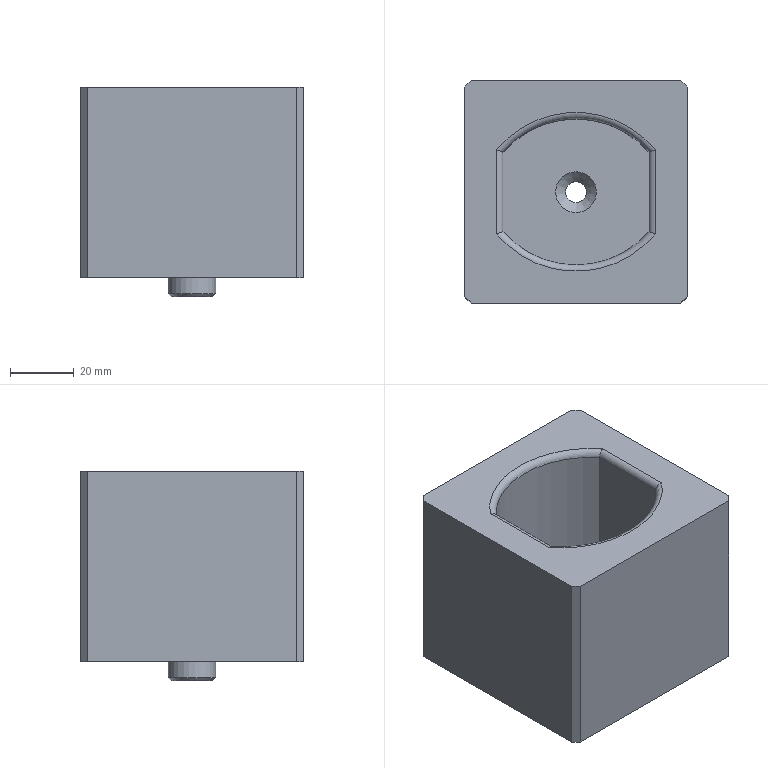NC program | NX | posted with a generic post | part box 70 x 70 x 66 mm
Whole program:
N10 G17 G21 G94 G90
(FLOOR_WALL , TOOL : D63)
N12 T01 M6
N14 G54
N16 G17 G0 G90 X-72.5 Y37.997 S6500 M3
N18 G43 Z30. H1
N20 Z3.
N22 G94 G1 Z0. F2500.
N24 X-69.5
N26 X69.5
N28 Y12.599
N30 X-69.5
N32 Y-12.8
N34 X69.5
N36 X72.5
N38 Z3.
N40 G0 Z30.
N42 M5
(DRILLING , TOOL : D8A45)
N44 T06 M6
N46 G54
N48 G17 G0 G90 X0. Y0. S5000 M3
N50 G43 Z30. H6
N52 G94 G81 G98 Z-3.4 F250. R3.
N54 G80
N56 G0 X0. Y0. Z30.
N58 M5
(DRILLING_COPY , TOOL : 6.6ZT)
N60 T16 M6
N62 G54
N64 G17 G0 G90 X0. Y0. S2000 M3
N66 G43 Z30. H16
N68 G94 G83 G98 Z-14.983 F250. Q2. R3.
N70 G80
N72 G0 X0. Y0. Z30.
N74 M5
(ZLEVEL_PROFILE , TOOL : D16)
N76 T22 M6
N78 G54
N80 G17 G0 G90 X-2.862 Y-43.15 S7500 M3
N82 G43 Z30. H22
N84 Z1.4
N86 G94 G1 X-33. Z-0.179 F1000.
N88 X-33.7 Z-0.216
N90 X-35.342 Y-42.838 Z-0.304
N92 X-36.886 Y-42.198 Z-0.391
N94 X-38.268 Y-41.258 Z-0.479
N96 X-41.258 Y-38.268 Z-0.701
N98 X-42.198 Y-36.886 Z-0.788
N100 X-42.838 Y-35.342 Z-0.876
N102 X-43.15 Y-33.7 Z-0.963
N104 Y-33. Z-1.
N106 Y33. F2500.
N108 G2 X-40.763 Y38.763 R8.15
N110 G1 X-38.763 Y40.763
N112 G2 X-33. Y43.15 R8.15
N114 G1 X33.
N116 G2 X38.763 Y40.763 R8.15
N118 G1 X40.763 Y38.763
N120 G2 X43.15 Y33. R8.15
N122 G1 Y-33.
N124 G2 X40.763 Y-38.763 R8.15
N126 G1 X38.763 Y-40.763
N128 G2 X33. Y-43.15 R8.15
N130 G1 X-33.
N132 G2 X-38.763 Y-40.763 R8.15
N134 G1 X-40.763 Y-38.763
N136 G2 X-43.15 Y-33. R8.15
N138 G1 Y24.29 Z-2.
N140 Y33.
N142 G2 X-40.763 Y38.763 R8.15
N144 G1 X-38.763 Y40.763
N146 G2 X-33. Y43.15 R8.15
N148 G1 X33.
N150 G2 X38.763 Y40.763 R8.15
N152 G1 X40.763 Y38.763
N154 G2 X43.15 Y33. R8.15
N156 G1 Y-33.
N158 G2 X40.763 Y-38.763 R8.15
N160 G1 X38.763 Y-40.763
N162 G2 X33. Y-43.15 R8.15
N164 G1 X-33.
N166 G2 X-38.763 Y-40.763 R8.15
N168 G1 X-40.763 Y-38.763
N170 G2 X-43.15 Y-33. R8.15
N172 G1 Y24.29 Z-3.
N174 Y33.
N176 G2 X-40.763 Y38.763 R8.15
N178 G1 X-38.763 Y40.763
N180 G2 X-33. Y43.15 R8.15
N182 G1 X33.
N184 G2 X38.763 Y40.763 R8.15
N186 G1 X40.763 Y38.763
N188 G2 X43.15 Y33. R8.15
N190 G1 Y-33.
N192 G2 X40.763 Y-38.763 R8.15
N194 G1 X38.763 Y-40.763
N196 G2 X33. Y-43.15 R8.15
N198 G1 X-33.
N200 G2 X-38.763 Y-40.763 R8.15
N202 G1 X-40.763 Y-38.763
N204 G2 X-43.15 Y-33. R8.15
N206 G1 Y24.29 Z-4.
N208 Y33.
N210 G2 X-40.763 Y38.763 R8.15
N212 G1 X-38.763 Y40.763
N214 G2 X-33. Y43.15 R8.15
N216 G1 X33.
N218 G2 X38.763 Y40.763 R8.15
N220 G1 X40.763 Y38.763
N222 G2 X43.15 Y33. R8.15
N224 G1 Y-33.
N226 G2 X40.763 Y-38.763 R8.15
N228 G1 X38.763 Y-40.763
N230 G2 X33. Y-43.15 R8.15
N232 G1 X-33.
N234 G2 X-38.763 Y-40.763 R8.15
N236 G1 X-40.763 Y-38.763
N238 G2 X-43.15 Y-33. R8.15
N240 G1 Y24.29 Z-5.
N242 Y33.
N244 G2 X-40.763 Y38.763 R8.15
N246 G1 X-38.763 Y40.763
N248 G2 X-33. Y43.15 R8.15
N250 G1 X33.
N252 G2 X38.763 Y40.763 R8.15
N254 G1 X40.763 Y38.763
N256 G2 X43.15 Y33. R8.15
N258 G1 Y-33.
N260 G2 X40.763 Y-38.763 R8.15
N262 G1 X38.763 Y-40.763
N264 G2 X33. Y-43.15 R8.15
N266 G1 X-33.
N268 G2 X-38.763 Y-40.763 R8.15
N270 G1 X-40.763 Y-38.763
N272 G2 X-43.15 Y-33. R8.15
N274 G1 Y24.29 Z-6.
N276 Y33.
N278 G2 X-40.763 Y38.763 R8.15
N280 G1 X-38.763 Y40.763
N282 G2 X-33. Y43.15 R8.15
N284 G1 X33.
N286 G2 X38.763 Y40.763 R8.15
N288 G1 X40.763 Y38.763
N290 G2 X43.15 Y33. R8.15
N292 G1 Y-33.
N294 G2 X40.763 Y-38.763 R8.15
N296 G1 X38.763 Y-40.763
N298 G2 X33. Y-43.15 R8.15
N300 G1 X-33.
N302 G2 X-38.763 Y-40.763 R8.15
N304 G1 X-40.763 Y-38.763
N306 G2 X-43.15 Y-33. R8.15
N308 G1 Y24.29 Z-7.
N310 Y33.
N312 G2 X-40.763 Y38.763 R8.15
N314 G1 X-38.763 Y40.763
N316 G2 X-33. Y43.15 R8.15
N318 G1 X33.
N320 G2 X38.763 Y40.763 R8.15
N322 G1 X40.763 Y38.763
N324 G2 X43.15 Y33. R8.15
N326 G1 Y-33.
N328 G2 X40.763 Y-38.763 R8.15
N330 G1 X38.763 Y-40.763
N332 G2 X33. Y-43.15 R8.15
N334 G1 X-33.
N336 G2 X-38.763 Y-40.763 R8.15
N338 G1 X-40.763 Y-38.763
N340 G2 X-43.15 Y-33. R8.15
N342 G1 Y24.29 Z-8.
N344 Y33.
N346 G2 X-40.763 Y38.763 R8.15
N348 G1 X-38.763 Y40.763
N350 G2 X-33. Y43.15 R8.15
N352 G1 X33.
N354 G2 X38.763 Y40.763 R8.15
N356 G1 X40.763 Y38.763
N358 G2 X43.15 Y33. R8.15
N360 G1 Y-33.
N362 G2 X40.763 Y-38.763 R8.15
N364 G1 X38.763 Y-40.763
N366 G2 X33. Y-43.15 R8.15
N368 G1 X-33.
N370 G2 X-38.763 Y-40.763 R8.15
N372 G1 X-40.763 Y-38.763
N374 G2 X-43.15 Y-33. R8.15
N376 G1 Y24.29 Z-9.
N378 Y33.
N380 G2 X-40.763 Y38.763 R8.15
N382 G1 X-38.763 Y40.763
N384 G2 X-33. Y43.15 R8.15
N386 G1 X33.
N388 G2 X38.763 Y40.763 R8.15
N390 G1 X40.763 Y38.763
N392 G2 X43.15 Y33. R8.15
N394 G1 Y-33.
N396 G2 X40.763 Y-38.763 R8.15
N398 G1 X38.763 Y-40.763
N400 G2 X33. Y-43.15 R8.15
N402 G1 X-33.
N404 G2 X-38.763 Y-40.763 R8.15
N406 G1 X-40.763 Y-38.763
N408 G2 X-43.15 Y-33. R8.15
N410 G1 Y24.29 Z-10.
N412 Y33.
N414 G2 X-40.763 Y38.763 R8.15
N416 G1 X-38.763 Y40.763
N418 G2 X-33. Y43.15 R8.15
N420 G1 X33.
N422 G2 X38.763 Y40.763 R8.15
N424 G1 X40.763 Y38.763
N426 G2 X43.15 Y33. R8.15
N428 G1 Y-33.
N430 G2 X40.763 Y-38.763 R8.15
N432 G1 X38.763 Y-40.763
N434 G2 X33. Y-43.15 R8.15
N436 G1 X-33.
N438 G2 X-38.763 Y-40.763 R8.15
N440 G1 X-40.763 Y-38.763
N442 G2 X-43.15 Y-33. R8.15
N444 G1 Y24.29 Z-11.
N446 Y33.
N448 G2 X-40.763 Y38.763 R8.15
N450 G1 X-38.763 Y40.763
N452 G2 X-33. Y43.15 R8.15
N454 G1 X33.
N456 G2 X38.763 Y40.763 R8.15
N458 G1 X40.763 Y38.763
N460 G2 X43.15 Y33. R8.15
N462 G1 Y-33.
N464 G2 X40.763 Y-38.763 R8.15
N466 G1 X38.763 Y-40.763
N468 G2 X33. Y-43.15 R8.15
N470 G1 X-33.
N472 G2 X-38.763 Y-40.763 R8.15
N474 G1 X-40.763 Y-38.763
N476 G2 X-43.15 Y-33. R8.15
N478 G1 Y24.29 Z-12.
N480 Y33.
N482 G2 X-40.763 Y38.763 R8.15
N484 G1 X-38.763 Y40.763
N486 G2 X-33. Y43.15 R8.15
N488 G1 X33.
N490 G2 X38.763 Y40.763 R8.15
N492 G1 X40.763 Y38.763
N494 G2 X43.15 Y33. R8.15
N496 G1 Y-33.
N498 G2 X40.763 Y-38.763 R8.15
N500 G1 X38.763 Y-40.763
N502 G2 X33. Y-43.15 R8.15
N504 G1 X-33.
N506 G2 X-38.763 Y-40.763 R8.15
N508 G1 X-40.763 Y-38.763
N510 G2 X-43.15 Y-33. R8.15
N512 G1 Y24.29 Z-13.
N514 Y33.
N516 G2 X-40.763 Y38.763 R8.15
N518 G1 X-38.763 Y40.763
N520 G2 X-33. Y43.15 R8.15
N522 G1 X33.
N524 G2 X38.763 Y40.763 R8.15
N526 G1 X40.763 Y38.763
N528 G2 X43.15 Y33. R8.15
N530 G1 Y-33.
N532 G2 X40.763 Y-38.763 R8.15
N534 G1 X38.763 Y-40.763
N536 G2 X33. Y-43.15 R8.15
N538 G1 X-33.
N540 G2 X-38.763 Y-40.763 R8.15
N542 G1 X-40.763 Y-38.763
N544 G2 X-43.15 Y-33. R8.15
N546 G1 Y24.29 Z-14.
N548 Y33.
N550 G2 X-40.763 Y38.763 R8.15
N552 G1 X-38.763 Y40.763
N554 G2 X-33. Y43.15 R8.15
N556 G1 X33.
N558 G2 X38.763 Y40.763 R8.15
N560 G1 X40.763 Y38.763
N562 G2 X43.15 Y33. R8.15
N564 G1 Y-33.
N566 G2 X40.763 Y-38.763 R8.15
N568 G1 X38.763 Y-40.763
N570 G2 X33. Y-43.15 R8.15
N572 G1 X-33.
N574 G2 X-38.763 Y-40.763 R8.15
N576 G1 X-40.763 Y-38.763
N578 G2 X-43.15 Y-33. R8.15
N580 G1 Y24.29 Z-15.
N582 Y33.
N584 G2 X-40.763 Y38.763 R8.15
N586 G1 X-38.763 Y40.763
N588 G2 X-33. Y43.15 R8.15
N590 G1 X33.
N592 G2 X38.763 Y40.763 R8.15
N594 G1 X40.763 Y38.763
N596 G2 X43.15 Y33. R8.15
N598 G1 Y-33.
N600 G2 X40.763 Y-38.763 R8.15
N602 G1 X38.763 Y-40.763
N604 G2 X33. Y-43.15 R8.15
N606 G1 X-33.
N608 G2 X-38.763 Y-40.763 R8.15
N610 G1 X-40.763 Y-38.763
N612 G2 X-43.15 Y-33. R8.15
N614 G1 Y24.29 Z-16.
N616 Y33.
N618 G2 X-40.763 Y38.763 R8.15
N620 G1 X-38.763 Y40.763
N622 G2 X-33. Y43.15 R8.15
N624 G1 X33.
N626 G2 X38.763 Y40.763 R8.15
N628 G1 X40.763 Y38.763
N630 G2 X43.15 Y33. R8.15
N632 G1 Y-33.
N634 G2 X40.763 Y-38.763 R8.15
N636 G1 X38.763 Y-40.763
N638 G2 X33. Y-43.15 R8.15
N640 G1 X-33.
N642 G2 X-38.763 Y-40.763 R8.15
N644 G1 X-40.763 Y-38.763
N646 G2 X-43.15 Y-33. R8.15
N648 G1 Y24.29 Z-17.
N650 Y33.
N652 G2 X-40.763 Y38.763 R8.15
N654 G1 X-38.763 Y40.763
N656 G2 X-33. Y43.15 R8.15
N658 G1 X33.
N660 G2 X38.763 Y40.763 R8.15
N662 G1 X40.763 Y38.763
N664 G2 X43.15 Y33. R8.15
N666 G1 Y-33.
N668 G2 X40.763 Y-38.763 R8.15
N670 G1 X38.763 Y-40.763
N672 G2 X33. Y-43.15 R8.15
N674 G1 X-33.
N676 G2 X-38.763 Y-40.763 R8.15
N678 G1 X-40.763 Y-38.763
N680 G2 X-43.15 Y-33. R8.15
N682 G1 Y24.29 Z-18.
N684 Y33.
N686 G2 X-40.763 Y38.763 R8.15
N688 G1 X-38.763 Y40.763
N690 G2 X-33. Y43.15 R8.15
N692 G1 X33.
N694 G2 X38.763 Y40.763 R8.15
N696 G1 X40.763 Y38.763
N698 G2 X43.15 Y33. R8.15
N700 G1 Y-33.
N702 G2 X40.763 Y-38.763 R8.15
N704 G1 X38.763 Y-40.763
N706 G2 X33. Y-43.15 R8.15
N708 G1 X-33.
N710 G2 X-38.763 Y-40.763 R8.15
N712 G1 X-40.763 Y-38.763
N714 G2 X-43.15 Y-33. R8.15
N716 G1 Y24.29 Z-19.
N718 Y33.
N720 G2 X-40.763 Y38.763 R8.15
N722 G1 X-38.763 Y40.763
N724 G2 X-33. Y43.15 R8.15
N726 G1 X33.
N728 G2 X38.763 Y40.763 R8.15
N730 G1 X40.763 Y38.763
N732 G2 X43.15 Y33. R8.15
N734 G1 Y-33.
N736 G2 X40.763 Y-38.763 R8.15
N738 G1 X38.763 Y-40.763
N740 G2 X33. Y-43.15 R8.15
N742 G1 X-33.
N744 G2 X-38.763 Y-40.763 R8.15
N746 G1 X-40.763 Y-38.763
N748 G2 X-43.15 Y-33. R8.15
N750 G1 Y24.29 Z-20.
N752 Y33.
N754 G2 X-40.763 Y38.763 R8.15
N756 G1 X-38.763 Y40.763
N758 G2 X-33. Y43.15 R8.15
N760 G1 X33.
N762 G2 X38.763 Y40.763 R8.15
N764 G1 X40.763 Y38.763
N766 G2 X43.15 Y33. R8.15
N768 G1 Y-33.
N770 G2 X40.763 Y-38.763 R8.15
N772 G1 X38.763 Y-40.763
N774 G2 X33. Y-43.15 R8.15
N776 G1 X-33.
N778 G2 X-38.763 Y-40.763 R8.15
N780 G1 X-40.763 Y-38.763
N782 G2 X-43.15 Y-33. R8.15
N784 G1 Y24.29 Z-21.
N786 Y33.
N788 G2 X-40.763 Y38.763 R8.15
N790 G1 X-38.763 Y40.763
N792 G2 X-33. Y43.15 R8.15
N794 G1 X33.
N796 G2 X38.763 Y40.763 R8.15
N798 G1 X40.763 Y38.763
N800 G2 X43.15 Y33. R8.15
N802 G1 Y-33.
N804 G2 X40.763 Y-38.763 R8.15
N806 G1 X38.763 Y-40.763
N808 G2 X33. Y-43.15 R8.15
N810 G1 X-33.
N812 G2 X-38.763 Y-40.763 R8.15
N814 G1 X-40.763 Y-38.763
N816 G2 X-43.15 Y-33. R8.15
N818 G1 Y24.29 Z-22.
N820 Y33.
N822 G2 X-40.763 Y38.763 R8.15
N824 G1 X-38.763 Y40.763
N826 G2 X-33. Y43.15 R8.15
N828 G1 X33.
N830 G2 X38.763 Y40.763 R8.15
N832 G1 X40.763 Y38.763
N834 G2 X43.15 Y33. R8.15
N836 G1 Y-33.
N838 G2 X40.763 Y-38.763 R8.15
N840 G1 X38.763 Y-40.763
N842 G2 X33. Y-43.15 R8.15
N844 G1 X-33.
N846 G2 X-38.763 Y-40.763 R8.15
N848 G1 X-40.763 Y-38.763
N850 G2 X-43.15 Y-33. R8.15
N852 G1 Y24.29 Z-23.
N854 Y33.
N856 G2 X-40.763 Y38.763 R8.15
N858 G1 X-38.763 Y40.763
N860 G2 X-33. Y43.15 R8.15
N862 G1 X33.
N864 G2 X38.763 Y40.763 R8.15
N866 G1 X40.763 Y38.763
N868 G2 X43.15 Y33. R8.15
N870 G1 Y-33.
N872 G2 X40.763 Y-38.763 R8.15
N874 G1 X38.763 Y-40.763
N876 G2 X33. Y-43.15 R8.15
N878 G1 X-33.
N880 G2 X-38.763 Y-40.763 R8.15
N882 G1 X-40.763 Y-38.763
N884 G2 X-43.15 Y-33. R8.15
N886 G1 Y24.29 Z-24.
N888 Y33.
N890 G2 X-40.763 Y38.763 R8.15
N892 G1 X-38.763 Y40.763
N894 G2 X-33. Y43.15 R8.15
N896 G1 X33.
N898 G2 X38.763 Y40.763 R8.15
N900 G1 X40.763 Y38.763
N902 G2 X43.15 Y33. R8.15
N904 G1 Y-33.
N906 G2 X40.763 Y-38.763 R8.15
N908 G1 X38.763 Y-40.763
N910 G2 X33. Y-43.15 R8.15
N912 G1 X-33.
N914 G2 X-38.763 Y-40.763 R8.15
N916 G1 X-40.763 Y-38.763
N918 G2 X-43.15 Y-33. R8.15
N920 G1 Y24.29 Z-25.
N922 Y33.
N924 G2 X-40.763 Y38.763 R8.15
N926 G1 X-38.763 Y40.763
N928 G2 X-33. Y43.15 R8.15
N930 G1 X33.
N932 G2 X38.763 Y40.763 R8.15
N934 G1 X40.763 Y38.763
N936 G2 X43.15 Y33. R8.15
N938 G1 Y-33.
N940 G2 X40.763 Y-38.763 R8.15
N942 G1 X38.763 Y-40.763
N944 G2 X33. Y-43.15 R8.15
N946 G1 X-33.
N948 G2 X-38.763 Y-40.763 R8.15
N950 G1 X-40.763 Y-38.763
N952 G2 X-43.15 Y-33. R8.15
N954 G1 Y24.29 Z-26.
N956 Y33.
N958 G2 X-40.763 Y38.763 R8.15
N960 G1 X-38.763 Y40.763
N962 G2 X-33. Y43.15 R8.15
N964 G1 X33.
N966 G2 X38.763 Y40.763 R8.15
N968 G1 X40.763 Y38.763
N970 G2 X43.15 Y33. R8.15
N972 G1 Y-33.
N974 G2 X40.763 Y-38.763 R8.15
N976 G1 X38.763 Y-40.763
N978 G2 X33. Y-43.15 R8.15
N980 G1 X-33.
N982 G2 X-38.763 Y-40.763 R8.15
N984 G1 X-40.763 Y-38.763
N986 G2 X-43.15 Y-33. R8.15
N988 G1 Y24.29 Z-27.
N990 Y33.
N992 G2 X-40.763 Y38.763 R8.15
N994 G1 X-38.763 Y40.763
N996 G2 X-33. Y43.15 R8.15
N998 G1 X33.
N1000 G2 X38.763 Y40.763 R8.15
N1002 G1 X40.763 Y38.763
N1004 G2 X43.15 Y33. R8.15
N1006 G1 Y-33.
N1008 G2 X40.763 Y-38.763 R8.15
N1010 G1 X38.763 Y-40.763
N1012 G2 X33. Y-43.15 R8.15
N1014 G1 X-33.
N1016 G2 X-38.763 Y-40.763 R8.15
N1018 G1 X-40.763 Y-38.763
N1020 G2 X-43.15 Y-33. R8.15
N1022 G1 Y24.29 Z-28.
N1024 Y33.
N1026 G2 X-40.763 Y38.763 R8.15
N1028 G1 X-38.763 Y40.763
N1030 G2 X-33. Y43.15 R8.15
N1032 G1 X33.
N1034 G2 X38.763 Y40.763 R8.15
N1036 G1 X40.763 Y38.763
N1038 G2 X43.15 Y33. R8.15
N1040 G1 Y-33.
N1042 G2 X40.763 Y-38.763 R8.15
N1044 G1 X38.763 Y-40.763
N1046 G2 X33. Y-43.15 R8.15
N1048 G1 X-33.
N1050 G2 X-38.763 Y-40.763 R8.15
N1052 G1 X-40.763 Y-38.763
N1054 G2 X-43.15 Y-33. R8.15
N1056 G1 Y24.29 Z-29.
N1058 Y33.
N1060 G2 X-40.763 Y38.763 R8.15
N1062 G1 X-38.763 Y40.763
N1064 G2 X-33. Y43.15 R8.15
N1066 G1 X33.
N1068 G2 X38.763 Y40.763 R8.15
N1070 G1 X40.763 Y38.763
N1072 G2 X43.15 Y33. R8.15
N1074 G1 Y-33.
N1076 G2 X40.763 Y-38.763 R8.15
N1078 G1 X38.763 Y-40.763
N1080 G2 X33. Y-43.15 R8.15
N1082 G1 X-33.
N1084 G2 X-38.763 Y-40.763 R8.15
N1086 G1 X-40.763 Y-38.763
N1088 G2 X-43.15 Y-33. R8.15
N1090 G1 Y24.29 Z-30.
N1092 Y33.
N1094 G2 X-40.763 Y38.763 R8.15
N1096 G1 X-38.763 Y40.763
N1098 G2 X-33. Y43.15 R8.15
N1100 G1 X33.
N1102 G2 X38.763 Y40.763 R8.15
N1104 G1 X40.763 Y38.763
N1106 G2 X43.15 Y33. R8.15
N1108 G1 Y-33.
N1110 G2 X40.763 Y-38.763 R8.15
N1112 G1 X38.763 Y-40.763
N1114 G2 X33. Y-43.15 R8.15
N1116 G1 X-33.
N1118 G2 X-38.763 Y-40.763 R8.15
N1120 G1 X-40.763 Y-38.763
N1122 G2 X-43.15 Y-33. R8.15
N1124 G1 Y24.29 Z-31.
N1126 Y33.
N1128 G2 X-40.763 Y38.763 R8.15
N1130 G1 X-38.763 Y40.763
N1132 G2 X-33. Y43.15 R8.15
N1134 G1 X33.
N1136 G2 X38.763 Y40.763 R8.15
N1138 G1 X40.763 Y38.763
N1140 G2 X43.15 Y33. R8.15
N1142 G1 Y-33.
N1144 G2 X40.763 Y-38.763 R8.15
N1146 G1 X38.763 Y-40.763
N1148 G2 X33. Y-43.15 R8.15
N1150 G1 X-33.
N1152 G2 X-38.763 Y-40.763 R8.15
N1154 G1 X-40.763 Y-38.763
N1156 G2 X-43.15 Y-33. R8.15
N1158 G1 Y24.29 Z-32.
N1160 Y33.
N1162 G2 X-40.763 Y38.763 R8.15
N1164 G1 X-38.763 Y40.763
N1166 G2 X-33. Y43.15 R8.15
N1168 G1 X33.
N1170 G2 X38.763 Y40.763 R8.15
N1172 G1 X40.763 Y38.763
N1174 G2 X43.15 Y33. R8.15
N1176 G1 Y-33.
N1178 G2 X40.763 Y-38.763 R8.15
N1180 G1 X38.763 Y-40.763
N1182 G2 X33. Y-43.15 R8.15
N1184 G1 X-33.
N1186 G2 X-38.763 Y-40.763 R8.15
N1188 G1 X-40.763 Y-38.763
N1190 G2 X-43.15 Y-33. R8.15
N1192 G1 Y24.29 Z-33.
N1194 Y33.
N1196 G2 X-40.763 Y38.763 R8.15
N1198 G1 X-38.763 Y40.763
N1200 G2 X-33. Y43.15 R8.15
N1202 G1 X33.
N1204 G2 X38.763 Y40.763 R8.15
N1206 G1 X40.763 Y38.763
N1208 G2 X43.15 Y33. R8.15
N1210 G1 Y-33.
N1212 G2 X40.763 Y-38.763 R8.15
N1214 G1 X38.763 Y-40.763
N1216 G2 X33. Y-43.15 R8.15
N1218 G1 X-33.
N1220 G2 X-38.763 Y-40.763 R8.15
N1222 G1 X-40.763 Y-38.763
N1224 G2 X-43.15 Y-33. R8.15
N1226 G1 Y24.29 Z-34.
N1228 Y33.
N1230 G2 X-40.763 Y38.763 R8.15
N1232 G1 X-38.763 Y40.763
N1234 G2 X-33. Y43.15 R8.15
N1236 G1 X33.
N1238 G2 X38.763 Y40.763 R8.15
N1240 G1 X40.763 Y38.763
N1242 G2 X43.15 Y33. R8.15
N1244 G1 Y-33.
N1246 G2 X40.763 Y-38.763 R8.15
N1248 G1 X38.763 Y-40.763
N1250 G2 X33. Y-43.15 R8.15
N1252 G1 X-33.
N1254 G2 X-38.763 Y-40.763 R8.15
N1256 G1 X-40.763 Y-38.763
N1258 G2 X-43.15 Y-33. R8.15
N1260 G1 Y24.29 Z-35.
N1262 Y33.
N1264 G2 X-40.763 Y38.763 R8.15
N1266 G1 X-38.763 Y40.763
N1268 G2 X-33. Y43.15 R8.15
N1270 G1 X33.
N1272 G2 X38.763 Y40.763 R8.15
N1274 G1 X40.763 Y38.763
N1276 G2 X43.15 Y33. R8.15
N1278 G1 Y-33.
N1280 G2 X40.763 Y-38.763 R8.15
N1282 G1 X38.763 Y-40.763
N1284 G2 X33. Y-43.15 R8.15
N1286 G1 X-33.
N1288 G2 X-38.763 Y-40.763 R8.15
N1290 G1 X-40.763 Y-38.763
N1292 G2 X-43.15 Y-33. R8.15
N1294 G1 Y24.29 Z-36.
N1296 Y33.
N1298 G2 X-40.763 Y38.763 R8.15
N1300 G1 X-38.763 Y40.763
N1302 G2 X-33. Y43.15 R8.15
N1304 G1 X33.
N1306 G2 X38.763 Y40.763 R8.15
N1308 G1 X40.763 Y38.763
N1310 G2 X43.15 Y33. R8.15
N1312 G1 Y-33.
N1314 G2 X40.763 Y-38.763 R8.15
N1316 G1 X38.763 Y-40.763
N1318 G2 X33. Y-43.15 R8.15
N1320 G1 X-33.
N1322 G2 X-38.763 Y-40.763 R8.15
N1324 G1 X-40.763 Y-38.763
N1326 G2 X-43.15 Y-33. R8.15
N1328 G1 Y24.29 Z-37.
N1330 Y33.
N1332 G2 X-40.763 Y38.763 R8.15
N1334 G1 X-38.763 Y40.763
N1336 G2 X-33. Y43.15 R8.15
N1338 G1 X33.
N1340 G2 X38.763 Y40.763 R8.15
N1342 G1 X40.763 Y38.763
N1344 G2 X43.15 Y33. R8.15
N1346 G1 Y-33.
N1348 G2 X40.763 Y-38.763 R8.15
N1350 G1 X38.763 Y-40.763
N1352 G2 X33. Y-43.15 R8.15
N1354 G1 X-33.
N1356 G2 X-38.763 Y-40.763 R8.15
N1358 G1 X-40.763 Y-38.763
N1360 G2 X-43.15 Y-33. R8.15
N1362 G1 Y24.29 Z-38.
N1364 Y33.
N1366 G2 X-40.763 Y38.763 R8.15
N1368 G1 X-38.763 Y40.763
N1370 G2 X-33. Y43.15 R8.15
N1372 G1 X33.
N1374 G2 X38.763 Y40.763 R8.15
N1376 G1 X40.763 Y38.763
N1378 G2 X43.15 Y33. R8.15
N1380 G1 Y-33.
N1382 G2 X40.763 Y-38.763 R8.15
N1384 G1 X38.763 Y-40.763
N1386 G2 X33. Y-43.15 R8.15
N1388 G1 X-33.
N1390 G2 X-38.763 Y-40.763 R8.15
N1392 G1 X-40.763 Y-38.763
N1394 G2 X-43.15 Y-33. R8.15
N1396 G1 Y24.29 Z-39.
N1398 Y33.
N1400 G2 X-40.763 Y38.763 R8.15
N1402 G1 X-38.763 Y40.763
N1404 G2 X-33. Y43.15 R8.15
N1406 G1 X33.
N1408 G2 X38.763 Y40.763 R8.15
N1410 G1 X40.763 Y38.763
N1412 G2 X43.15 Y33. R8.15
N1414 G1 Y-33.
N1416 G2 X40.763 Y-38.763 R8.15
N1418 G1 X38.763 Y-40.763
N1420 G2 X33. Y-43.15 R8.15
N1422 G1 X-33.
N1424 G2 X-38.763 Y-40.763 R8.15
N1426 G1 X-40.763 Y-38.763
N1428 G2 X-43.15 Y-33. R8.15
N1430 G1 Y24.29 Z-40.
N1432 Y33.
N1434 G2 X-40.763 Y38.763 R8.15
N1436 G1 X-38.763 Y40.763
N1438 G2 X-33. Y43.15 R8.15
N1440 G1 X33.
N1442 G2 X38.763 Y40.763 R8.15
N1444 G1 X40.763 Y38.763
N1446 G2 X43.15 Y33. R8.15
N1448 G1 Y-33.
N1450 G2 X40.763 Y-38.763 R8.15
N1452 G1 X38.763 Y-40.763
N1454 G2 X33. Y-43.15 R8.15
N1456 G1 X-33.
N1458 G2 X-38.763 Y-40.763 R8.15
N1460 G1 X-40.763 Y-38.763
N1462 G2 X-43.15 Y-33. R8.15
N1464 G1 Y24.29 Z-41.
N1466 Y33.
N1468 G2 X-40.763 Y38.763 R8.15
N1470 G1 X-38.763 Y40.763
N1472 G2 X-33. Y43.15 R8.15
N1474 G1 X33.
N1476 G2 X38.763 Y40.763 R8.15
N1478 G1 X40.763 Y38.763
N1480 G2 X43.15 Y33. R8.15
N1482 G1 Y-33.
N1484 G2 X40.763 Y-38.763 R8.15
N1486 G1 X38.763 Y-40.763
N1488 G2 X33. Y-43.15 R8.15
N1490 G1 X-33.
N1492 G2 X-38.763 Y-40.763 R8.15
N1494 G1 X-40.763 Y-38.763
N1496 G2 X-43.15 Y-33. R8.15
N1498 G1 Y24.29 Z-42.
N1500 Y33.
N1502 G2 X-40.763 Y38.763 R8.15
N1504 G1 X-38.763 Y40.763
N1506 G2 X-33. Y43.15 R8.15
N1508 G1 X33.
N1510 G2 X38.763 Y40.763 R8.15
N1512 G1 X40.763 Y38.763
N1514 G2 X43.15 Y33. R8.15
N1516 G1 Y-33.
N1518 G2 X40.763 Y-38.763 R8.15
N1520 G1 X38.763 Y-40.763
N1522 G2 X33. Y-43.15 R8.15
N1524 G1 X-33.
N1526 G2 X-38.763 Y-40.763 R8.15
N1528 G1 X-40.763 Y-38.763
N1530 G2 X-43.15 Y-33. R8.15
N1532 G1 Y24.29 Z-43.
N1534 Y33.
N1536 G2 X-40.763 Y38.763 R8.15
N1538 G1 X-38.763 Y40.763
N1540 G2 X-33. Y43.15 R8.15
N1542 G1 X33.
N1544 G2 X38.763 Y40.763 R8.15
N1546 G1 X40.763 Y38.763
N1548 G2 X43.15 Y33. R8.15
N1550 G1 Y-33.
N1552 G2 X40.763 Y-38.763 R8.15
N1554 G1 X38.763 Y-40.763
N1556 G2 X33. Y-43.15 R8.15
N1558 G1 X-33.
N1560 G2 X-38.763 Y-40.763 R8.15
N1562 G1 X-40.763 Y-38.763
N1564 G2 X-43.15 Y-33. R8.15
N1566 G1 Y24.29 Z-44.
N1568 Y33.
N1570 G2 X-40.763 Y38.763 R8.15
N1572 G1 X-38.763 Y40.763
N1574 G2 X-33. Y43.15 R8.15
N1576 G1 X33.
N1578 G2 X38.763 Y40.763 R8.15
N1580 G1 X40.763 Y38.763
N1582 G2 X43.15 Y33. R8.15
N1584 G1 Y-33.
N1586 G2 X40.763 Y-38.763 R8.15
N1588 G1 X38.763 Y-40.763
N1590 G2 X33. Y-43.15 R8.15
N1592 G1 X-33.
N1594 G2 X-38.763 Y-40.763 R8.15
N1596 G1 X-40.763 Y-38.763
N1598 G2 X-43.15 Y-33. R8.15
N1600 G1 Y24.29 Z-45.
N1602 Y33.
N1604 G2 X-40.763 Y38.763 R8.15
N1606 G1 X-38.763 Y40.763
N1608 G2 X-33. Y43.15 R8.15
N1610 G1 X33.
N1612 G2 X38.763 Y40.763 R8.15
N1614 G1 X40.763 Y38.763
N1616 G2 X43.15 Y33. R8.15
N1618 G1 Y-33.
N1620 G2 X40.763 Y-38.763 R8.15
N1622 G1 X38.763 Y-40.763
N1624 G2 X33. Y-43.15 R8.15
N1626 G1 X-33.
N1628 G2 X-38.763 Y-40.763 R8.15
N1630 G1 X-40.763 Y-38.763
N1632 G2 X-43.15 Y-33. R8.15
N1634 G1 Y24.29 Z-46.
N1636 Y33.
N1638 G2 X-40.763 Y38.763 R8.15
N1640 G1 X-38.763 Y40.763
N1642 G2 X-33. Y43.15 R8.15
N1644 G1 X33.
N1646 G2 X38.763 Y40.763 R8.15
N1648 G1 X40.763 Y38.763
N1650 G2 X43.15 Y33. R8.15
N1652 G1 Y-33.
N1654 G2 X40.763 Y-38.763 R8.15
N1656 G1 X38.763 Y-40.763
N1658 G2 X33. Y-43.15 R8.15
N1660 G1 X-33.
N1662 G2 X-38.763 Y-40.763 R8.15
N1664 G1 X-40.763 Y-38.763
N1666 G2 X-43.15 Y-33. R8.15
N1668 G1 Y24.29 Z-47.
N1670 Y33.
N1672 G2 X-40.763 Y38.763 R8.15
N1674 G1 X-38.763 Y40.763
N1676 G2 X-33. Y43.15 R8.15
N1678 G1 X33.
N1680 G2 X38.763 Y40.763 R8.15
N1682 G1 X40.763 Y38.763
N1684 G2 X43.15 Y33. R8.15
N1686 G1 Y-33.
N1688 G2 X40.763 Y-38.763 R8.15
N1690 G1 X38.763 Y-40.763
N1692 G2 X33. Y-43.15 R8.15
N1694 G1 X-33.
N1696 G2 X-38.763 Y-40.763 R8.15
N1698 G1 X-40.763 Y-38.763
N1700 G2 X-43.15 Y-33. R8.15
N1702 G1 Y24.29 Z-48.
N1704 Y33.
N1706 G2 X-40.763 Y38.763 R8.15
N1708 G1 X-38.763 Y40.763
N1710 G2 X-33. Y43.15 R8.15
N1712 G1 X33.
N1714 G2 X38.763 Y40.763 R8.15
N1716 G1 X40.763 Y38.763
N1718 G2 X43.15 Y33. R8.15
N1720 G1 Y-33.
N1722 G2 X40.763 Y-38.763 R8.15
N1724 G1 X38.763 Y-40.763
N1726 G2 X33. Y-43.15 R8.15
N1728 G1 X-33.
N1730 G2 X-38.763 Y-40.763 R8.15
N1732 G1 X-40.763 Y-38.763
N1734 G2 X-43.15 Y-33. R8.15
N1736 G1 Y24.29 Z-49.
N1738 Y33.
N1740 G2 X-40.763 Y38.763 R8.15
N1742 G1 X-38.763 Y40.763
N1744 G2 X-33. Y43.15 R8.15
N1746 G1 X33.
N1748 G2 X38.763 Y40.763 R8.15
N1750 G1 X40.763 Y38.763
N1752 G2 X43.15 Y33. R8.15
N1754 G1 Y-33.
N1756 G2 X40.763 Y-38.763 R8.15
N1758 G1 X38.763 Y-40.763
N1760 G2 X33. Y-43.15 R8.15
N1762 G1 X-33.
N1764 G2 X-38.763 Y-40.763 R8.15
N1766 G1 X-40.763 Y-38.763
N1768 G2 X-43.15 Y-33. R8.15
N1770 G1 Y24.29 Z-50.
N1772 Y33.
N1774 G2 X-40.763 Y38.763 R8.15
N1776 G1 X-38.763 Y40.763
N1778 G2 X-33. Y43.15 R8.15
N1780 G1 X33.
N1782 G2 X38.763 Y40.763 R8.15
N1784 G1 X40.763 Y38.763
N1786 G2 X43.15 Y33. R8.15
N1788 G1 Y-33.
N1790 G2 X40.763 Y-38.763 R8.15
N1792 G1 X38.763 Y-40.763
N1794 G2 X33. Y-43.15 R8.15
N1796 G1 X-33.
N1798 G2 X-38.763 Y-40.763 R8.15
N1800 G1 X-40.763 Y-38.763
N1802 G2 X-43.15 Y-33. R8.15
N1804 G1 Y24.29 Z-51.
N1806 Y33.
N1808 G2 X-40.763 Y38.763 R8.15
N1810 G1 X-38.763 Y40.763
N1812 G2 X-33. Y43.15 R8.15
N1814 G1 X33.
N1816 G2 X38.763 Y40.763 R8.15
N1818 G1 X40.763 Y38.763
N1820 G2 X43.15 Y33. R8.15
N1822 G1 Y-33.
N1824 G2 X40.763 Y-38.763 R8.15
N1826 G1 X38.763 Y-40.763
N1828 G2 X33. Y-43.15 R8.15
N1830 G1 X-33.
N1832 G2 X-38.763 Y-40.763 R8.15
N1834 G1 X-40.763 Y-38.763
N1836 G2 X-43.15 Y-33. R8.15
N1838 G1 Y24.29 Z-52.
N1840 Y33.
N1842 G2 X-40.763 Y38.763 R8.15
N1844 G1 X-38.763 Y40.763
N1846 G2 X-33. Y43.15 R8.15
N1848 G1 X33.
N1850 G2 X38.763 Y40.763 R8.15
N1852 G1 X40.763 Y38.763
N1854 G2 X43.15 Y33. R8.15
N1856 G1 Y-33.
N1858 G2 X40.763 Y-38.763 R8.15
N1860 G1 X38.763 Y-40.763
N1862 G2 X33. Y-43.15 R8.15
N1864 G1 X-33.
N1866 G2 X-38.763 Y-40.763 R8.15
N1868 G1 X-40.763 Y-38.763
N1870 G2 X-43.15 Y-33. R8.15
N1872 G1 Y24.29 Z-53.
N1874 Y33.
N1876 G2 X-40.763 Y38.763 R8.15
N1878 G1 X-38.763 Y40.763
N1880 G2 X-33. Y43.15 R8.15
N1882 G1 X33.
N1884 G2 X38.763 Y40.763 R8.15
N1886 G1 X40.763 Y38.763
N1888 G2 X43.15 Y33. R8.15
N1890 G1 Y-33.
N1892 G2 X40.763 Y-38.763 R8.15
N1894 G1 X38.763 Y-40.763
N1896 G2 X33. Y-43.15 R8.15
N1898 G1 X-33.
N1900 G2 X-38.763 Y-40.763 R8.15
N1902 G1 X-40.763 Y-38.763
N1904 G2 X-43.15 Y-33. R8.15
N1906 G1 Y24.29 Z-54.
N1908 Y33.
N1910 G2 X-40.763 Y38.763 R8.15
N1912 G1 X-38.763 Y40.763
N1914 G2 X-33. Y43.15 R8.15
N1916 G1 X33.
N1918 G2 X38.763 Y40.763 R8.15
N1920 G1 X40.763 Y38.763
N1922 G2 X43.15 Y33. R8.15
N1924 G1 Y-33.
N1926 G2 X40.763 Y-38.763 R8.15
N1928 G1 X38.763 Y-40.763
N1930 G2 X33. Y-43.15 R8.15
N1932 G1 X-33.
N1934 G2 X-38.763 Y-40.763 R8.15
N1936 G1 X-40.763 Y-38.763
N1938 G2 X-43.15 Y-33. R8.15
N1940 G1 Y24.29 Z-55.
N1942 Y33.
N1944 G2 X-40.763 Y38.763 R8.15
N1946 G1 X-38.763 Y40.763
N1948 G2 X-33. Y43.15 R8.15
N1950 G1 X33.
N1952 G2 X38.763 Y40.763 R8.15
N1954 G1 X40.763 Y38.763
N1956 G2 X43.15 Y33. R8.15
N1958 G1 Y-33.
N1960 G2 X40.763 Y-38.763 R8.15
N1962 G1 X38.763 Y-40.763
N1964 G2 X33. Y-43.15 R8.15
N1966 G1 X-33.
N1968 G2 X-38.763 Y-40.763 R8.15
N1970 G1 X-40.763 Y-38.763
N1972 G2 X-43.15 Y-33. R8.15
N1974 G1 Y24.29 Z-56.
N1976 Y33.
N1978 G2 X-40.763 Y38.763 R8.15
N1980 G1 X-38.763 Y40.763
N1982 G2 X-33. Y43.15 R8.15
N1984 G1 X33.
N1986 G2 X38.763 Y40.763 R8.15
N1988 G1 X40.763 Y38.763
N1990 G2 X43.15 Y33. R8.15
N1992 G1 Y-33.
N1994 G2 X40.763 Y-38.763 R8.15
N1996 G1 X38.763 Y-40.763
N1998 G2 X33. Y-43.15 R8.15
N2000 G1 X-33.
N2002 G2 X-38.763 Y-40.763 R8.15
N2004 G1 X-40.763 Y-38.763
N2006 G2 X-43.15 Y-33. R8.15
N2008 G1 Y24.29 Z-57.
N2010 Y33.
N2012 G2 X-40.763 Y38.763 R8.15
N2014 G1 X-38.763 Y40.763
N2016 G2 X-33. Y43.15 R8.15
N2018 G1 X33.
N2020 G2 X38.763 Y40.763 R8.15
N2022 G1 X40.763 Y38.763
N2024 G2 X43.15 Y33. R8.15
N2026 G1 Y-33.
N2028 G2 X40.763 Y-38.763 R8.15
N2030 G1 X38.763 Y-40.763
N2032 G2 X33. Y-43.15 R8.15
N2034 G1 X-33.
N2036 G2 X-38.763 Y-40.763 R8.15
N2038 G1 X-40.763 Y-38.763
N2040 G2 X-43.15 Y-33. R8.15
N2042 G1 Y24.29 Z-58.
N2044 Y33.
N2046 G2 X-40.763 Y38.763 R8.15
N2048 G1 X-38.763 Y40.763
N2050 G2 X-33. Y43.15 R8.15
N2052 G1 X33.
N2054 G2 X38.763 Y40.763 R8.15
N2056 G1 X40.763 Y38.763
N2058 G2 X43.15 Y33. R8.15
N2060 G1 Y-33.
N2062 G2 X40.763 Y-38.763 R8.15
N2064 G1 X38.763 Y-40.763
N2066 G2 X33. Y-43.15 R8.15
N2068 G1 X-33.
N2070 G2 X-38.763 Y-40.763 R8.15
N2072 G1 X-40.763 Y-38.763
N2074 G2 X-43.15 Y-33. R8.15
N2076 G1 Y24.29 Z-59.
N2078 Y33.
N2080 G2 X-40.763 Y38.763 R8.15
N2082 G1 X-38.763 Y40.763
N2084 G2 X-33. Y43.15 R8.15
N2086 G1 X33.
N2088 G2 X38.763 Y40.763 R8.15
N2090 G1 X40.763 Y38.763
N2092 G2 X43.15 Y33. R8.15
N2094 G1 Y-33.
N2096 G2 X40.763 Y-38.763 R8.15
N2098 G1 X38.763 Y-40.763
N2100 G2 X33. Y-43.15 R8.15
N2102 G1 X-33.
N2104 G2 X-38.763 Y-40.763 R8.15
N2106 G1 X-40.763 Y-38.763
N2108 G2 X-43.15 Y-33. R8.15
N2110 G1 Y24.29 Z-60.
N2112 Y33.
N2114 G2 X-40.763 Y38.763 R8.15
N2116 G1 X-38.763 Y40.763
N2118 G2 X-33. Y43.15 R8.15
N2120 G1 X33.
N2122 G2 X38.763 Y40.763 R8.15
N2124 G1 X40.763 Y38.763
N2126 G2 X43.15 Y33. R8.15
N2128 G1 Y-33.
N2130 G2 X40.763 Y-38.763 R8.15
N2132 G1 X38.763 Y-40.763
N2134 G2 X33. Y-43.15 R8.15
N2136 G1 X-33.
N2138 G2 X-38.763 Y-40.763 R8.15
N2140 G1 X-40.763 Y-38.763
N2142 G2 X-43.15 Y-33. R8.15
N2144 G1 Y24.29 Z-61.
N2146 Y33.
N2148 G2 X-40.763 Y38.763 R8.15
N2150 G1 X-38.763 Y40.763
N2152 G2 X-33. Y43.15 R8.15
N2154 G1 X33.
N2156 G2 X38.763 Y40.763 R8.15
N2158 G1 X40.763 Y38.763
N2160 G2 X43.15 Y33. R8.15
N2162 G1 Y-33.
N2164 G2 X40.763 Y-38.763 R8.15
N2166 G1 X38.763 Y-40.763
N2168 G2 X33. Y-43.15 R8.15
N2170 G1 X-33.
N2172 G2 X-38.763 Y-40.763 R8.15
N2174 G1 X-40.763 Y-38.763
N2176 G2 X-43.15 Y-33. R8.15
N2178 G1 Y24.29 Z-62.
N2180 Y33.
N2182 G2 X-40.763 Y38.763 R8.15
N2184 G1 X-38.763 Y40.763
N2186 G2 X-33. Y43.15 R8.15
N2188 G1 X33.
N2190 G2 X38.763 Y40.763 R8.15
N2192 G1 X40.763 Y38.763
N2194 G2 X43.15 Y33. R8.15
N2196 G1 Y-33.
N2198 G2 X40.763 Y-38.763 R8.15
N2200 G1 X38.763 Y-40.763
N2202 G2 X33. Y-43.15 R8.15
N2204 G1 X-33.
N2206 G2 X-38.763 Y-40.763 R8.15
N2208 G1 X-40.763 Y-38.763
N2210 G2 X-43.15 Y-33. R8.15
N2212 G1 Y24.29 Z-63.
N2214 Y33.
N2216 G2 X-40.763 Y38.763 R8.15
N2218 G1 X-38.763 Y40.763
N2220 G2 X-33. Y43.15 R8.15
N2222 G1 X33.
N2224 G2 X38.763 Y40.763 R8.15
N2226 G1 X40.763 Y38.763
N2228 G2 X43.15 Y33. R8.15
N2230 G1 Y-33.
N2232 G2 X40.763 Y-38.763 R8.15
N2234 G1 X38.763 Y-40.763
N2236 G2 X33. Y-43.15 R8.15
N2238 G1 X-33.
N2240 G2 X-38.763 Y-40.763 R8.15
N2242 G1 X-40.763 Y-38.763
N2244 G2 X-43.15 Y-33. R8.15
N2246 G1 Y24.29 Z-64.
N2248 Y33.
N2250 G2 X-40.763 Y38.763 R8.15
N2252 G1 X-38.763 Y40.763
N2254 G2 X-33. Y43.15 R8.15
N2256 G1 X33.
N2258 G2 X38.763 Y40.763 R8.15
N2260 G1 X40.763 Y38.763
N2262 G2 X43.15 Y33. R8.15
N2264 G1 Y-33.
N2266 G2 X40.763 Y-38.763 R8.15
N2268 G1 X38.763 Y-40.763
N2270 G2 X33. Y-43.15 R8.15
N2272 G1 X-33.
N2274 G2 X-38.763 Y-40.763 R8.15
N2276 G1 X-40.763 Y-38.763
N2278 G2 X-43.15 Y-33. R8.15
N2280 G1 Y24.29 Z-65.
N2282 Y33.
N2284 G2 X-40.763 Y38.763 R8.15
N2286 G1 X-38.763 Y40.763
N2288 G2 X-33. Y43.15 R8.15
N2290 G1 X33.
N2292 G2 X38.763 Y40.763 R8.15
N2294 G1 X40.763 Y38.763
N2296 G2 X43.15 Y33. R8.15
N2298 G1 Y-33.
N2300 G2 X40.763 Y-38.763 R8.15
N2302 G1 X38.763 Y-40.763
N2304 G2 X33. Y-43.15 R8.15
N2306 G1 X-33.
N2308 G2 X-38.763 Y-40.763 R8.15
N2310 G1 X-40.763 Y-38.763
N2312 G2 X-43.15 Y-33. R8.15
N2314 G1 Y24.29 Z-66.
N2316 Y33.
N2318 G2 X-40.763 Y38.763 R8.15
N2320 G1 X-38.763 Y40.763
N2322 G2 X-33. Y43.15 R8.15
N2324 G1 X33.
N2326 G2 X38.763 Y40.763 R8.15
N2328 G1 X40.763 Y38.763
N2330 G2 X43.15 Y33. R8.15
N2332 G1 Y-33.
N2334 G2 X40.763 Y-38.763 R8.15
N2336 G1 X38.763 Y-40.763
N2338 G2 X33. Y-43.15 R8.15
N2340 G1 X-33.
N2342 G2 X-38.763 Y-40.763 R8.15
N2344 G1 X-40.763 Y-38.763
N2346 G2 X-43.15 Y-33. R8.15
N2348 G1 Y24.29
N2350 Z-64.6
N2352 G0 Z30.
(ZLEVEL_PROFILE_COPY , TOOL : D16)
N2354 X-45.895 Y-35.595
N2356 Z-15.
N2358 G1 Z-16.5 F1000.
N2360 X-43.8 Y-34.386
N2362 G3 X-43. Y-33. R1.6
N2364 G1 Y33. F850.
N2366 G2 X-40.657 Y38.657 R8.
N2368 G1 X-38.657 Y40.657
N2370 G2 X-33. Y43. R8.
N2372 G1 X33.
N2374 G2 X38.657 Y40.657 R8.
N2376 G1 X40.657 Y38.657
N2378 G2 X43. Y33. R8.
N2380 G1 Y-33.
N2382 G2 X40.657 Y-38.657 R8.
N2384 G1 X38.657 Y-40.657
N2386 G2 X33. Y-43. R8.
N2388 G1 X-33.
N2390 G2 X-38.657 Y-40.657 R8.
N2392 G1 X-40.657 Y-38.657
N2394 G2 X-43. Y-33. R8.
N2396 G3 X-43.8 Y-31.614 R1.6
N2398 G1 X-46.2 Y-30.229
N2400 Z-15.
N2402 G0 X-45.895 Y-35.595 Z-31.5
N2404 G1 Z-33. F1000.
N2406 X-43.8 Y-34.386
N2408 G3 X-43. Y-33. R1.6
N2410 G1 Y33. F850.
N2412 G2 X-40.657 Y38.657 R8.
N2414 G1 X-38.657 Y40.657
N2416 G2 X-33. Y43. R8.
N2418 G1 X33.
N2420 G2 X38.657 Y40.657 R8.
N2422 G1 X40.657 Y38.657
N2424 G2 X43. Y33. R8.
N2426 G1 Y-33.
N2428 G2 X40.657 Y-38.657 R8.
N2430 G1 X38.657 Y-40.657
N2432 G2 X33. Y-43. R8.
N2434 G1 X-33.
N2436 G2 X-38.657 Y-40.657 R8.
N2438 G1 X-40.657 Y-38.657
N2440 G2 X-43. Y-33. R8.
N2442 G3 X-43.8 Y-31.614 R1.6
N2444 G1 X-46.2 Y-30.229
N2446 Z-31.5
N2448 G0 X-45.895 Y-35.595 Z-48.
N2450 G1 Z-49.5 F1000.
N2452 X-43.8 Y-34.386
N2454 G3 X-43. Y-33. R1.6
N2456 G1 Y33. F850.
N2458 G2 X-40.657 Y38.657 R8.
N2460 G1 X-38.657 Y40.657
N2462 G2 X-33. Y43. R8.
N2464 G1 X33.
N2466 G2 X38.657 Y40.657 R8.
N2468 G1 X40.657 Y38.657
N2470 G2 X43. Y33. R8.
N2472 G1 Y-33.
N2474 G2 X40.657 Y-38.657 R8.
N2476 G1 X38.657 Y-40.657
N2478 G2 X33. Y-43. R8.
N2480 G1 X-33.
N2482 G2 X-38.657 Y-40.657 R8.
N2484 G1 X-40.657 Y-38.657
N2486 G2 X-43. Y-33. R8.
N2488 G3 X-43.8 Y-31.614 R1.6
N2490 G1 X-46.2 Y-30.229
N2492 Z-48.
N2494 G0 X-45.895 Y-35.595 Z-64.5
N2496 G1 Z-66. F1000.
N2498 X-43.8 Y-34.386
N2500 G3 X-43. Y-33. R1.6
N2502 G1 Y33. F850.
N2504 G2 X-40.657 Y38.657 R8.
N2506 G1 X-38.657 Y40.657
N2508 G2 X-33. Y43. R8.
N2510 G1 X33.
N2512 G2 X38.657 Y40.657 R8.
N2514 G1 X40.657 Y38.657
N2516 G2 X43. Y33. R8.
N2518 G1 Y-33.
N2520 G2 X40.657 Y-38.657 R8.
N2522 G1 X38.657 Y-40.657
N2524 G2 X33. Y-43. R8.
N2526 G1 X-33.
N2528 G2 X-38.657 Y-40.657 R8.
N2530 G1 X-40.657 Y-38.657
N2532 G2 X-43. Y-33. R8.
N2534 G3 X-43.8 Y-31.614 R1.6
N2536 G1 X-46.2 Y-30.229
N2538 Z-64.5
N2540 G0 Z30.
N2542 M5
(FLOOR_WALL_1 , TOOL : D10)
N2544 T04 M6
N2546 G54
N2548 G17 G0 G90 X-11.922 Y41.5 S7500 M3
N2550 G43 Z30. H4
N2552 Z0.525
N2554 G94 G1 Z-0.975 F1000.
N2556 X-8.458 Y35.5
N2558 G3 X-7.592 Y35. R1.
N2560 G1 X33. F2500.
N2562 X35. Y33.
N2564 Y-33.
N2566 X33. Y-35.
N2568 X-33.
N2570 X-35. Y-33.
N2572 Y33.
N2574 X-33. Y35.
N2576 X-7.592
N2578 Y28.
N2580 X28.
N2582 Y-28.
N2584 X-28.
N2586 Y28.
N2588 X-7.592
N2590 Y21.
N2592 X21.
N2594 Y1.184
N2596 X14.
N2598 G3 X1.184 Y14. R14.05
N2600 G1 X14.
N2602 Y1.184
N2604 X21.
N2606 Y-21.
N2608 X1.184
N2610 Y-14.
N2612 G3 X14. Y-1.184 R14.05
N2614 G1 Y-14.
N2616 X1.184
N2618 Y-21.
N2620 X-21.
N2622 Y-1.184
N2624 X-14.
N2626 G3 X-1.184 Y-14. R14.05
N2628 G1 X-14.
N2630 Y-1.184
N2632 X-21.
N2634 Y21.
N2636 X-7.592
N2638 Y14.
N2640 X-1.184
N2642 G3 X-14. Y1.184 R14.05
N2644 G1 X-12.605 Y1.066
N2646 G2 X1.066 Y12.605 R12.65
N2648 X-12.605 Y1.066 R-12.65
N2650 G1 X-14. Y1.184
N2652 Y14.
N2654 X-7.592
N2656 G3 X-6.726 Y14.5 R1.
N2658 G1 Z0.525
N2660 G0 X-11.922 Y41.5 Z-0.45
N2662 G1 Z-1.95 F1000.
N2664 X-8.458 Y35.5
N2666 G3 X-7.592 Y35. R1.
N2668 G1 X33. F2500.
N2670 X35. Y33.
N2672 Y-33.
N2674 X33. Y-35.
N2676 X-33.
N2678 X-35. Y-33.
N2680 Y33.
N2682 X-33. Y35.
N2684 X-7.592
N2686 Y28.
N2688 X28.
N2690 Y-28.
N2692 X-28.
N2694 Y28.
N2696 X-7.592
N2698 Y21.
N2700 X21.
N2702 Y1.184
N2704 X14.
N2706 G3 X1.184 Y14. R14.05
N2708 G1 X14.
N2710 Y1.184
N2712 X21.
N2714 Y-21.
N2716 X1.184
N2718 Y-14.
N2720 G3 X14. Y-1.184 R14.05
N2722 G1 Y-14.
N2724 X1.184
N2726 Y-21.
N2728 X-21.
N2730 Y-1.184
N2732 X-14.
N2734 G3 X-1.184 Y-14. R14.05
N2736 G1 X-14.
N2738 Y-1.184
N2740 X-21.
N2742 Y21.
N2744 X-7.592
N2746 Y14.
N2748 X-1.184
N2750 G3 X-14. Y1.184 R14.05
N2752 G1 X-12.605 Y1.066
N2754 G2 X1.066 Y12.605 R12.65
N2756 X-12.605 Y1.066 R-12.65
N2758 G1 X-14. Y1.184
N2760 Y14.
N2762 X-7.592
N2764 G3 X-6.726 Y14.5 R1.
N2766 G1 Z-0.45
N2768 G0 X-11.922 Y41.5 Z-1.425
N2770 G1 Z-2.925 F1000.
N2772 X-8.458 Y35.5
N2774 G3 X-7.592 Y35. R1.
N2776 G1 X33. F2500.
N2778 X35. Y33.
N2780 Y-33.
N2782 X33. Y-35.
N2784 X-33.
N2786 X-35. Y-33.
N2788 Y33.
N2790 X-33. Y35.
N2792 X-7.592
N2794 Y28.
N2796 X28.
N2798 Y-28.
N2800 X-28.
N2802 Y28.
N2804 X-7.592
N2806 Y21.
N2808 X21.
N2810 Y1.184
N2812 X14.
N2814 G3 X1.184 Y14. R14.05
N2816 G1 X14.
N2818 Y1.184
N2820 X21.
N2822 Y-21.
N2824 X1.184
N2826 Y-14.
N2828 G3 X14. Y-1.184 R14.05
N2830 G1 Y-14.
N2832 X1.184
N2834 Y-21.
N2836 X-21.
N2838 Y-1.184
N2840 X-14.
N2842 G3 X-1.184 Y-14. R14.05
N2844 G1 X-14.
N2846 Y-1.184
N2848 X-21.
N2850 Y21.
N2852 X-7.592
N2854 Y14.
N2856 X-1.184
N2858 G3 X-14. Y1.184 R14.05
N2860 G1 X-12.605 Y1.066
N2862 G2 X1.066 Y12.605 R12.65
N2864 X-12.605 Y1.066 R-12.65
N2866 G1 X-14. Y1.184
N2868 Y14.
N2870 X-7.592
N2872 G3 X-6.726 Y14.5 R1.
N2874 G1 Z-1.425
N2876 G0 X-11.922 Y41.5 Z-2.4
N2878 G1 Z-3.9 F1000.
N2880 X-8.458 Y35.5
N2882 G3 X-7.592 Y35. R1.
N2884 G1 X33. F2500.
N2886 X35. Y33.
N2888 Y-33.
N2890 X33. Y-35.
N2892 X-33.
N2894 X-35. Y-33.
N2896 Y33.
N2898 X-33. Y35.
N2900 X-7.592
N2902 Y28.
N2904 X28.
N2906 Y-28.
N2908 X-28.
N2910 Y28.
N2912 X-7.592
N2914 Y21.
N2916 X21.
N2918 Y1.184
N2920 X14.
N2922 G3 X1.184 Y14. R14.05
N2924 G1 X14.
N2926 Y1.184
N2928 X21.
N2930 Y-21.
N2932 X1.184
N2934 Y-14.
N2936 G3 X14. Y-1.184 R14.05
N2938 G1 Y-14.
N2940 X1.184
N2942 Y-21.
N2944 X-21.
N2946 Y-1.184
N2948 X-14.
N2950 G3 X-1.184 Y-14. R14.05
N2952 G1 X-14.
N2954 Y-1.184
N2956 X-21.
N2958 Y21.
N2960 X-7.592
N2962 Y14.
N2964 X-1.184
N2966 G3 X-14. Y1.184 R14.05
N2968 G1 X-12.605 Y1.066
N2970 G2 X1.066 Y12.605 R12.65
N2972 X-12.605 Y1.066 R-12.65
N2974 G1 X-14. Y1.184
N2976 Y14.
N2978 X-7.592
N2980 G3 X-6.726 Y14.5 R1.
N2982 G1 Z-2.4
N2984 G0 X-11.922 Y41.5 Z-3.375
N2986 G1 Z-4.875 F1000.
N2988 X-8.458 Y35.5
N2990 G3 X-7.592 Y35. R1.
N2992 G1 X33. F2500.
N2994 X35. Y33.
N2996 Y-33.
N2998 X33. Y-35.
N3000 X-33.
N3002 X-35. Y-33.
N3004 Y33.
N3006 X-33. Y35.
N3008 X-7.592
N3010 Y28.
N3012 X28.
N3014 Y-28.
N3016 X-28.
N3018 Y28.
N3020 X-7.592
N3022 Y21.
N3024 X21.
N3026 Y1.184
N3028 X14.
N3030 G3 X1.184 Y14. R14.05
N3032 G1 X14.
N3034 Y1.184
N3036 X21.
N3038 Y-21.
N3040 X1.184
N3042 Y-14.
N3044 G3 X14. Y-1.184 R14.05
N3046 G1 Y-14.
N3048 X1.184
N3050 Y-21.
N3052 X-21.
N3054 Y-1.184
N3056 X-14.
N3058 G3 X-1.184 Y-14. R14.05
N3060 G1 X-14.
N3062 Y-1.184
N3064 X-21.
N3066 Y21.
N3068 X-7.592
N3070 Y14.
N3072 X-1.184
N3074 G3 X-14. Y1.184 R14.05
N3076 G1 X-12.605 Y1.066
N3078 G2 X1.066 Y12.605 R12.65
N3080 X-12.605 Y1.066 R-12.65
N3082 G1 X-14. Y1.184
N3084 Y14.
N3086 X-7.592
N3088 G3 X-6.726 Y14.5 R1.
N3090 G1 Z-3.375
N3092 G0 X-11.922 Y41.5 Z-4.35
N3094 G1 Z-5.85 F1000.
N3096 X-8.458 Y35.5
N3098 G3 X-7.592 Y35. R1.
N3100 G1 X33. F2500.
N3102 X35. Y33.
N3104 Y-33.
N3106 X33. Y-35.
N3108 X-33.
N3110 X-35. Y-33.
N3112 Y33.
N3114 X-33. Y35.
N3116 X-7.592
N3118 Y28.
N3120 X28.
N3122 Y-28.
N3124 X-28.
N3126 Y28.
N3128 X-7.592
N3130 Y21.
N3132 X21.
N3134 Y1.184
N3136 X14.
N3138 G3 X1.184 Y14. R14.05
N3140 G1 X14.
N3142 Y1.184
N3144 X21.
N3146 Y-21.
N3148 X1.184
N3150 Y-14.
N3152 G3 X14. Y-1.184 R14.05
N3154 G1 Y-14.
N3156 X1.184
N3158 Y-21.
N3160 X-21.
N3162 Y-1.184
N3164 X-14.
N3166 G3 X-1.184 Y-14. R14.05
N3168 G1 X-14.
N3170 Y-1.184
N3172 X-21.
N3174 Y21.
N3176 X-7.592
N3178 Y14.
N3180 X-1.184
N3182 G3 X-14. Y1.184 R14.05
N3184 G1 X-12.605 Y1.066
N3186 G2 X1.066 Y12.605 R12.65
N3188 X-12.605 Y1.066 R-12.65
N3190 G1 X-14. Y1.184
N3192 Y14.
N3194 X-7.592
N3196 G3 X-6.726 Y14.5 R1.
N3198 G1 Z-4.35
N3200 G0 Z30.
(FLOOR_WALL_1_COPY , TOOL : D10)
N3202 X-41.165 Y36.015
N3204 Z-4.5
N3206 G1 Z-6. F1000.
N3208 X-40.866 Y35.497
N3210 G3 X-40. Y34.997 R1.
N3212 G1 X40.
N3214 Y28.397
N3216 X-40.
N3218 Y21.798
N3220 X40.
N3222 Y15.198
N3224 X-40.
N3226 Y8.598
N3228 X-9.75
N3230 G3 X-12.845 Y1.999 R13.
N3232 G1 X-40.
N3234 Y-4.601
N3236 X-12.158
N3238 G3 X-6.598 Y-11.201 R13.
N3240 G1 X-40.
N3242 G2 X-40.866 Y-10.701 R1.
N3244 G1 X-41.5 Y-9.603
N3246 Z-4.5
N3248 G0 Z-2.
N3250 G1 X-9.75 Y8.598 F8000.
N3252 G0 Z-4.5
N3254 G1 Z-6. F1000.
N3256 G2 X9.75 Y8.598 R13.
N3258 G1 X40.
N3260 Y1.999
N3262 X12.845
N3264 G2 X12.158 Y-4.601 R13.
N3266 G1 X40.
N3268 Y-11.201
N3270 X6.598
N3272 Z-4.5
N3274 G0 Z30.
N3276 X-41.5 Y-16.203
N3278 Z-4.5
N3280 G1 Z-6.
N3282 X-40.866 Y-17.301
N3284 G3 X-40. Y-17.801 R1.
N3286 G1 X40.
N3288 Y-24.4
N3290 X-40.
N3292 Y-31.
N3294 X40.
N3296 G3 X40.866 Y-30.5 R1.
N3298 G1 X41.5 Y-29.402
N3300 Z-4.5
N3302 G0 Z-2.
N3304 G1 X14.403 Y1.676 F8000.
N3306 G0 Z-4.5
N3308 G1 Z-6. F1000.
N3310 X13. Y0.866
N3312 G3 X12.5 Y0. R1.
N3314 G2 X0. Y-12.5 R12.5
N3316 X12.5 Y0. R-12.5
N3318 G3 X13. Y-0.866 R1.
N3320 G1 X14.403 Y-1.676
N3322 Z-4.5
N3324 G0 Z30.
N3326 M5
(PLANAR_MILL , TOOL : D8A45)
N3328 T06 M6
N3330 G54
N3332 G17 G0 G90 X-12. Y0. S7500 M3
N3334 G43 Z30. H6
N3336 Z1.5
N3338 G94 G1 Z-1.5 F1250.
N3340 X-8.
N3342 G2 X0. Y8. R8.
N3344 X-8. Y0. R-8.
N3346 G1 X-12.
N3348 Z1.5
N3350 G0 Z30.
(PLANAR_MILL_COPY , TOOL : D8A45)
N3352 X-40.3
N3354 Z-4.5
N3356 G1 Z-7.5
N3358 X-36.3
N3360 Y33.
N3362 G2 X-35.919 Y33.919 R1.3
N3364 G1 X-33.919 Y35.919
N3366 G2 X-33. Y36.3 R1.3
N3368 G1 X33.
N3370 G2 X33.919 Y35.919 R1.3
N3372 G1 X35.919 Y33.919
N3374 G2 X36.3 Y33. R1.3
N3376 G1 Y-33.
N3378 G2 X35.919 Y-33.919 R1.3
N3380 G1 X33.919 Y-35.919
N3382 G2 X33. Y-36.3 R1.3
N3384 G1 X-33.
N3386 G2 X-33.919 Y-35.919 R1.3
N3388 G1 X-35.919 Y-33.919
N3390 G2 X-36.3 Y-33. R1.3
N3392 G1 Y0.
N3394 X-40.3
N3396 Z-4.5
N3398 G0 Z30.
N3400 M5
N3402 M2